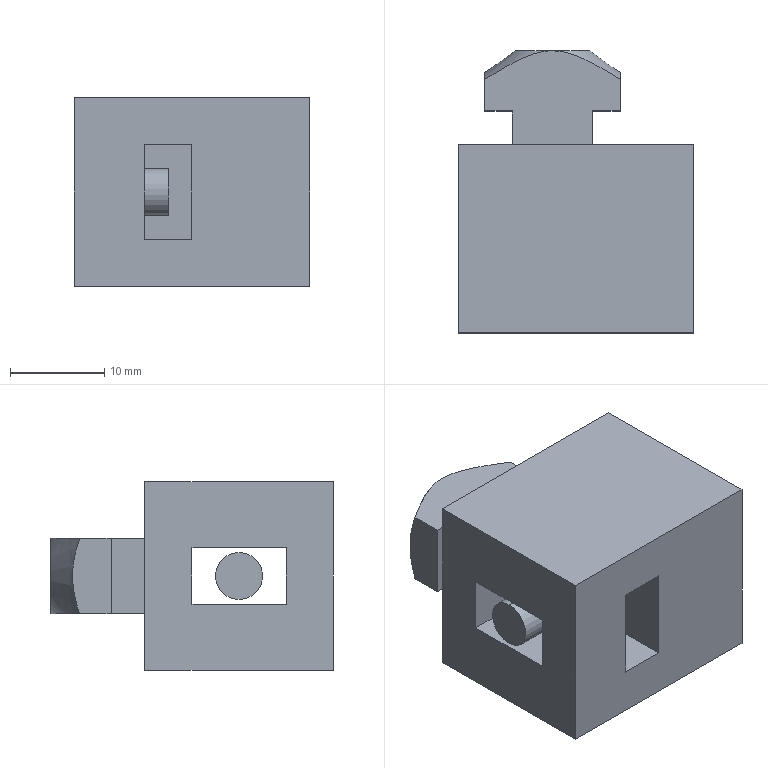Part | SolidWorks | features ICE 12, Draft 5, BaseBody 1 | 2 solids | 86 faces | box 25 x 30 x 20 mm | volume 9047 mm3 | plane 63 | spline 19 | cone 2 | cylinder 2 | commonest cylinder face diameters 5 x2